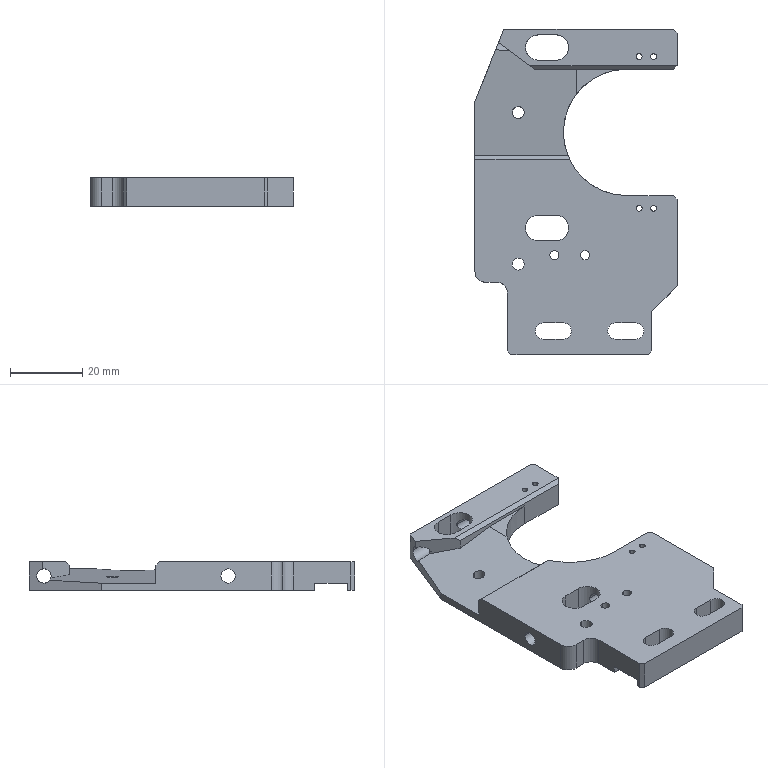Part | 1 solid | 73 faces | box 56 x 90 x 8 mm | volume 23118 mm3 | plane 38 | cylinder 35 | commonest cylinder face diameters 1.6 x8 4 x8 2.5 x4 3.3 x4 4.5 x4 7 x4